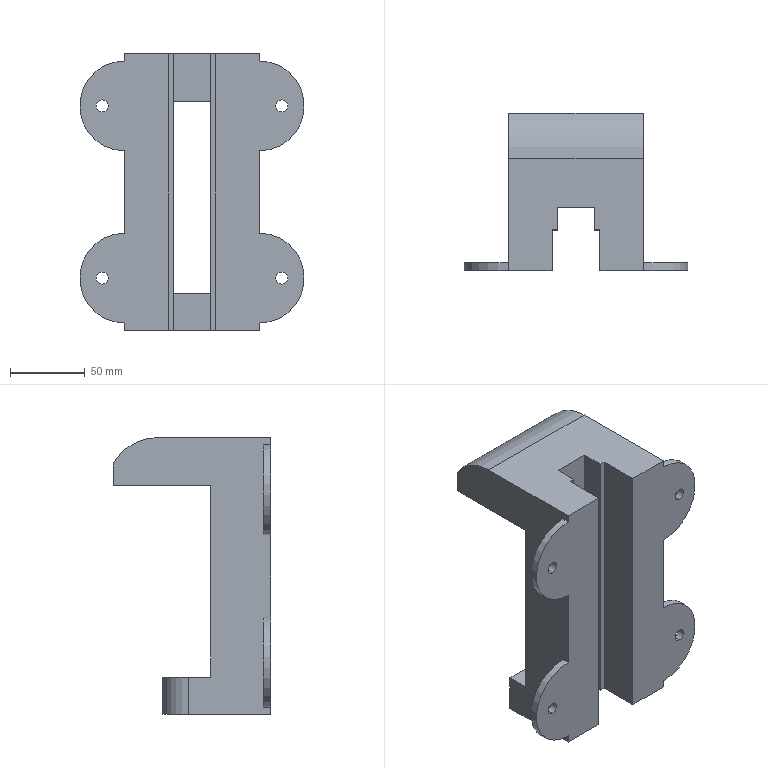Part | SolidWorks | features ICE 3, Extrusion 1, Helix 1, HoleWzd 1, SweepCut 1 | 1 solid | 82 faces | box 150 x 105 x 185 mm | volume 685281 mm3 | cylinder 48 | plane 27 | cone 4 | spline 3 | commonest cylinder face diameters 12 x26 8 x8 5 x4 6 x4 60 x4 34 x1